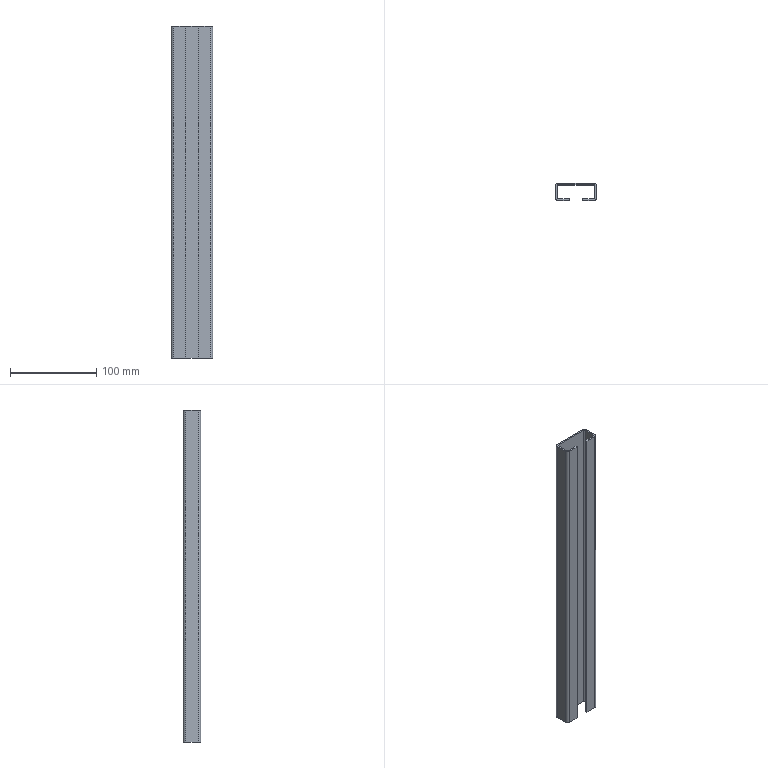Part | 1 solid | 38 faces | box 48 x 20 x 385 mm | volume 83596 mm3 | plane 30 | cylinder 8 | commonest cylinder face diameters 2 x4 6 x4
STEP:
#1=CARTESIAN_POINT('',(-24.,-17.,192.5));
#2=VERTEX_POINT('',#1);
#3=CARTESIAN_POINT('',(-22.,-17.,192.5));
#4=VERTEX_POINT('',#3);
#5=CARTESIAN_POINT('',(-24.,-17.,192.5));
#6=DIRECTION('',(1.,0.,0.));
#7=VECTOR('',#6,1000.);
#8=LINE('',#5,#7);
#9=EDGE_CURVE('',#2,#4,#8,.T.);
#10=ORIENTED_EDGE('',*,*,#9,.F.);
#11=CARTESIAN_POINT('',(-21.,-20.,192.5));
#12=VERTEX_POINT('',#11);
#13=CARTESIAN_POINT('',(-21.,-17.,192.5));
#14=DIRECTION('',(0.,0.,-1.));
#15=DIRECTION('',(1.,0.,0.));
#16=AXIS2_PLACEMENT_3D('',#13,#14,#15);
#17=CIRCLE('',#16,3.);
#18=EDGE_CURVE('',#12,#2,#17,.T.);
#19=ORIENTED_EDGE('',*,*,#18,.F.);
#20=CARTESIAN_POINT('',(-21.,-18.,192.5));
#21=VERTEX_POINT('',#20);
#22=CARTESIAN_POINT('',(-21.,-18.,192.5));
#23=DIRECTION('',(0.,-1.,0.));
#24=VECTOR('',#23,1000.);
#25=LINE('',#22,#24);
#26=EDGE_CURVE('',#21,#12,#25,.T.);
#27=ORIENTED_EDGE('',*,*,#26,.F.);
#28=CARTESIAN_POINT('',(-21.,-17.,192.5));
#29=DIRECTION('',(0.,0.,-1.));
#30=DIRECTION('',(1.,0.,0.));
#31=AXIS2_PLACEMENT_3D('',#28,#29,#30);
#32=CIRCLE('',#31,1.);
#33=EDGE_CURVE('',#21,#4,#32,.T.);
#34=ORIENTED_EDGE('',*,*,#33,.T.);
#35=EDGE_LOOP('',(#10,#19,#27,#34));
#36=FACE_OUTER_BOUND('',#35,.T.);
#37=CARTESIAN_POINT('',(-24.,-17.,192.5));
#38=DIRECTION('',(0.,0.,1.));
#39=DIRECTION('',(1.,0.,0.));
#40=AXIS2_PLACEMENT_3D('',#37,#38,#39);
#41=PLANE('',#40);
#42=ADVANCED_FACE('',(#36),#41,.T.);
#43=CARTESIAN_POINT('',(-24.,-3.,192.5));
#44=VERTEX_POINT('',#43);
#45=CARTESIAN_POINT('',(-24.,-20.,192.5));
#46=DIRECTION('',(0.,1.,0.));
#47=VECTOR('',#46,1000.);
#48=LINE('',#45,#47);
#49=EDGE_CURVE('',#2,#44,#48,.T.);
#50=ORIENTED_EDGE('',*,*,#49,.F.);
#51=ORIENTED_EDGE('',*,*,#9,.T.);
#52=CARTESIAN_POINT('',(-22.,-3.,192.5));
#53=VERTEX_POINT('',#52);
#54=CARTESIAN_POINT('',(-22.,-20.,192.5));
#55=DIRECTION('',(0.,1.,0.));
#56=VECTOR('',#55,1000.);
#57=LINE('',#54,#56);
#58=EDGE_CURVE('',#4,#53,#57,.T.);
#59=ORIENTED_EDGE('',*,*,#58,.T.);
#60=CARTESIAN_POINT('',(-22.,-3.,192.5));
#61=DIRECTION('',(-1.,0.,0.));
#62=VECTOR('',#61,1000.);
#63=LINE('',#60,#62);
#64=EDGE_CURVE('',#53,#44,#63,.T.);
#65=ORIENTED_EDGE('',*,*,#64,.T.);
#66=EDGE_LOOP('',(#50,#51,#59,#65));
#67=FACE_OUTER_BOUND('',#66,.T.);
#68=CARTESIAN_POINT('',(-21.,-18.,192.5));
#69=DIRECTION('',(0.,0.,1.));
#70=DIRECTION('',(1.,0.,0.));
#71=AXIS2_PLACEMENT_3D('',#68,#69,#70);
#72=PLANE('',#71);
#73=ADVANCED_FACE('',(#67),#72,.T.);
#74=CARTESIAN_POINT('',(-21.,-20.,-192.5));
#75=VERTEX_POINT('',#74);
#76=CARTESIAN_POINT('',(-21.,-18.,-192.5));
#77=VERTEX_POINT('',#76);
#78=CARTESIAN_POINT('',(-21.,-20.,-192.5));
#79=DIRECTION('',(0.,1.,0.));
#80=VECTOR('',#79,1000.);
#81=LINE('',#78,#80);
#82=EDGE_CURVE('',#75,#77,#81,.T.);
#83=ORIENTED_EDGE('',*,*,#82,.F.);
#84=CARTESIAN_POINT('',(-24.,-17.,-192.5));
#85=VERTEX_POINT('',#84);
#86=CARTESIAN_POINT('',(-21.,-17.,-192.5));
#87=DIRECTION('',(0.,0.,-1.));
#88=DIRECTION('',(1.,0.,0.));
#89=AXIS2_PLACEMENT_3D('',#86,#87,#88);
#90=CIRCLE('',#89,3.);
#91=EDGE_CURVE('',#75,#85,#90,.T.);
#92=ORIENTED_EDGE('',*,*,#91,.T.);
#93=CARTESIAN_POINT('',(-22.,-17.,-192.5));
#94=VERTEX_POINT('',#93);
#95=CARTESIAN_POINT('',(-22.,-17.,-192.5));
#96=DIRECTION('',(-1.,0.,0.));
#97=VECTOR('',#96,1000.);
#98=LINE('',#95,#97);
#99=EDGE_CURVE('',#94,#85,#98,.T.);
#100=ORIENTED_EDGE('',*,*,#99,.F.);
#101=CARTESIAN_POINT('',(-21.,-17.,-192.5));
#102=DIRECTION('',(0.,0.,-1.));
#103=DIRECTION('',(1.,0.,0.));
#104=AXIS2_PLACEMENT_3D('',#101,#102,#103);
#105=CIRCLE('',#104,1.);
#106=EDGE_CURVE('',#77,#94,#105,.T.);
#107=ORIENTED_EDGE('',*,*,#106,.F.);
#108=EDGE_LOOP('',(#83,#92,#100,#107));
#109=FACE_OUTER_BOUND('',#108,.T.);
#110=CARTESIAN_POINT('',(-21.,-20.,-192.5));
#111=DIRECTION('',(0.,0.,-1.));
#112=DIRECTION('',(-1.,0.,0.));
#113=AXIS2_PLACEMENT_3D('',#110,#111,#112);
#114=PLANE('',#113);
#115=ADVANCED_FACE('',(#109),#114,.T.);
#116=CARTESIAN_POINT('',(-8.,-20.,-192.5));
#117=VERTEX_POINT('',#116);
#118=CARTESIAN_POINT('',(-8.,-20.,-192.5));
#119=DIRECTION('',(-1.,0.,0.));
#120=VECTOR('',#119,1000.);
#121=LINE('',#118,#120);
#122=EDGE_CURVE('',#117,#75,#121,.T.);
#123=ORIENTED_EDGE('',*,*,#122,.T.);
#124=ORIENTED_EDGE('',*,*,#82,.T.);
#125=CARTESIAN_POINT('',(-8.,-18.,-192.5));
#126=VERTEX_POINT('',#125);
#127=CARTESIAN_POINT('',(-8.,-18.,-192.5));
#128=DIRECTION('',(-1.,0.,0.));
#129=VECTOR('',#128,1000.);
#130=LINE('',#127,#129);
#131=EDGE_CURVE('',#126,#77,#130,.T.);
#132=ORIENTED_EDGE('',*,*,#131,.F.);
#133=CARTESIAN_POINT('',(-8.,-18.,-192.5));
#134=DIRECTION('',(0.,-1.,0.));
#135=VECTOR('',#134,1000.);
#136=LINE('',#133,#135);
#137=EDGE_CURVE('',#126,#117,#136,.T.);
#138=ORIENTED_EDGE('',*,*,#137,.T.);
#139=EDGE_LOOP('',(#123,#124,#132,#138));
#140=FACE_OUTER_BOUND('',#139,.T.);
#141=CARTESIAN_POINT('',(-22.,-17.,-192.5));
#142=DIRECTION('',(0.,0.,-1.));
#143=DIRECTION('',(-1.,0.,0.));
#144=AXIS2_PLACEMENT_3D('',#141,#142,#143);
#145=PLANE('',#144);
#146=ADVANCED_FACE('',(#140),#145,.T.);
#147=CARTESIAN_POINT('',(-21.,0.,192.5));
#148=VERTEX_POINT('',#147);
#149=CARTESIAN_POINT('',(-21.,-2.,192.5));
#150=VERTEX_POINT('',#149);
#151=CARTESIAN_POINT('',(-21.,0.,192.5));
#152=DIRECTION('',(0.,-1.,0.));
#153=VECTOR('',#152,1000.);
#154=LINE('',#151,#153);
#155=EDGE_CURVE('',#148,#150,#154,.T.);
#156=ORIENTED_EDGE('',*,*,#155,.F.);
#157=CARTESIAN_POINT('',(-21.,-3.,192.5));
#158=DIRECTION('',(0.,0.,-1.));
#159=DIRECTION('',(1.,0.,0.));
#160=AXIS2_PLACEMENT_3D('',#157,#158,#159);
#161=CIRCLE('',#160,3.);
#162=EDGE_CURVE('',#44,#148,#161,.T.);
#163=ORIENTED_EDGE('',*,*,#162,.F.);
#164=ORIENTED_EDGE('',*,*,#64,.F.);
#165=CARTESIAN_POINT('',(-21.,-3.,192.5));
#166=DIRECTION('',(0.,0.,-1.));
#167=DIRECTION('',(1.,0.,0.));
#168=AXIS2_PLACEMENT_3D('',#165,#166,#167);
#169=CIRCLE('',#168,1.);
#170=EDGE_CURVE('',#53,#150,#169,.T.);
#171=ORIENTED_EDGE('',*,*,#170,.T.);
#172=EDGE_LOOP('',(#156,#163,#164,#171));
#173=FACE_OUTER_BOUND('',#172,.T.);
#174=CARTESIAN_POINT('',(-21.,0.,192.5));
#175=DIRECTION('',(0.,0.,1.));
#176=DIRECTION('',(1.,0.,0.));
#177=AXIS2_PLACEMENT_3D('',#174,#175,#176);
#178=PLANE('',#177);
#179=ADVANCED_FACE('',(#173),#178,.T.);
#180=CARTESIAN_POINT('',(21.,0.,192.5));
#181=VERTEX_POINT('',#180);
#182=CARTESIAN_POINT('',(-24.,0.,192.5));
#183=DIRECTION('',(1.,0.,0.));
#184=VECTOR('',#183,1000.);
#185=LINE('',#182,#184);
#186=EDGE_CURVE('',#148,#181,#185,.T.);
#187=ORIENTED_EDGE('',*,*,#186,.F.);
#188=ORIENTED_EDGE('',*,*,#155,.T.);
#189=CARTESIAN_POINT('',(21.,-2.,192.5));
#190=VERTEX_POINT('',#189);
#191=CARTESIAN_POINT('',(-24.,-2.,192.5));
#192=DIRECTION('',(1.,0.,0.));
#193=VECTOR('',#192,1000.);
#194=LINE('',#191,#193);
#195=EDGE_CURVE('',#150,#190,#194,.T.);
#196=ORIENTED_EDGE('',*,*,#195,.T.);
#197=CARTESIAN_POINT('',(21.,-2.,192.5));
#198=DIRECTION('',(0.,1.,0.));
#199=VECTOR('',#198,1000.);
#200=LINE('',#197,#199);
#201=EDGE_CURVE('',#190,#181,#200,.T.);
#202=ORIENTED_EDGE('',*,*,#201,.T.);
#203=EDGE_LOOP('',(#187,#188,#196,#202));
#204=FACE_OUTER_BOUND('',#203,.T.);
#205=CARTESIAN_POINT('',(-22.,-3.,192.5));
#206=DIRECTION('',(0.,0.,1.));
#207=DIRECTION('',(1.,0.,0.));
#208=AXIS2_PLACEMENT_3D('',#205,#206,#207);
#209=PLANE('',#208);
#210=ADVANCED_FACE('',(#204),#209,.T.);
#211=CARTESIAN_POINT('',(-24.,-3.,-192.5));
#212=VERTEX_POINT('',#211);
#213=CARTESIAN_POINT('',(-22.,-3.,-192.5));
#214=VERTEX_POINT('',#213);
#215=CARTESIAN_POINT('',(-24.,-3.,-192.5));
#216=DIRECTION('',(1.,0.,0.));
#217=VECTOR('',#216,1000.);
#218=LINE('',#215,#217);
#219=EDGE_CURVE('',#212,#214,#218,.T.);
#220=ORIENTED_EDGE('',*,*,#219,.F.);
#221=CARTESIAN_POINT('',(-21.,0.,-192.5));
#222=VERTEX_POINT('',#221);
#223=CARTESIAN_POINT('',(-21.,-3.,-192.5));
#224=DIRECTION('',(0.,0.,-1.));
#225=DIRECTION('',(1.,0.,0.));
#226=AXIS2_PLACEMENT_3D('',#223,#224,#225);
#227=CIRCLE('',#226,3.);
#228=EDGE_CURVE('',#212,#222,#227,.T.);
#229=ORIENTED_EDGE('',*,*,#228,.T.);
#230=CARTESIAN_POINT('',(-21.,-2.,-192.5));
#231=VERTEX_POINT('',#230);
#232=CARTESIAN_POINT('',(-21.,-2.,-192.5));
#233=DIRECTION('',(0.,1.,0.));
#234=VECTOR('',#233,1000.);
#235=LINE('',#232,#234);
#236=EDGE_CURVE('',#231,#222,#235,.T.);
#237=ORIENTED_EDGE('',*,*,#236,.F.);
#238=CARTESIAN_POINT('',(-21.,-3.,-192.5));
#239=DIRECTION('',(0.,0.,-1.));
#240=DIRECTION('',(1.,0.,0.));
#241=AXIS2_PLACEMENT_3D('',#238,#239,#240);
#242=CIRCLE('',#241,1.);
#243=EDGE_CURVE('',#214,#231,#242,.T.);
#244=ORIENTED_EDGE('',*,*,#243,.F.);
#245=EDGE_LOOP('',(#220,#229,#237,#244));
#246=FACE_OUTER_BOUND('',#245,.T.);
#247=CARTESIAN_POINT('',(-24.,-3.,-192.5));
#248=DIRECTION('',(0.,0.,-1.));
#249=DIRECTION('',(-1.,0.,0.));
#250=AXIS2_PLACEMENT_3D('',#247,#248,#249);
#251=PLANE('',#250);
#252=ADVANCED_FACE('',(#246),#251,.T.);
#253=CARTESIAN_POINT('',(-24.,-20.,-192.5));
#254=DIRECTION('',(0.,1.,0.));
#255=VECTOR('',#254,1000.);
#256=LINE('',#253,#255);
#257=EDGE_CURVE('',#85,#212,#256,.T.);
#258=ORIENTED_EDGE('',*,*,#257,.T.);
#259=ORIENTED_EDGE('',*,*,#219,.T.);
#260=CARTESIAN_POINT('',(-22.,-20.,-192.5));
#261=DIRECTION('',(0.,1.,0.));
#262=VECTOR('',#261,1000.);
#263=LINE('',#260,#262);
#264=EDGE_CURVE('',#94,#214,#263,.T.);
#265=ORIENTED_EDGE('',*,*,#264,.F.);
#266=ORIENTED_EDGE('',*,*,#99,.T.);
#267=EDGE_LOOP('',(#258,#259,#265,#266));
#268=FACE_OUTER_BOUND('',#267,.T.);
#269=CARTESIAN_POINT('',(-21.,-2.,-192.5));
#270=DIRECTION('',(0.,0.,-1.));
#271=DIRECTION('',(-1.,0.,0.));
#272=AXIS2_PLACEMENT_3D('',#269,#270,#271);
#273=PLANE('',#272);
#274=ADVANCED_FACE('',(#268),#273,.T.);
#275=CARTESIAN_POINT('',(24.,-3.,192.5));
#276=VERTEX_POINT('',#275);
#277=CARTESIAN_POINT('',(22.,-3.,192.5));
#278=VERTEX_POINT('',#277);
#279=CARTESIAN_POINT('',(24.,-3.,192.5));
#280=DIRECTION('',(-1.,0.,0.));
#281=VECTOR('',#280,1000.);
#282=LINE('',#279,#281);
#283=EDGE_CURVE('',#276,#278,#282,.T.);
#284=ORIENTED_EDGE('',*,*,#283,.F.);
#285=CARTESIAN_POINT('',(21.,-3.,192.5));
#286=DIRECTION('',(0.,0.,-1.));
#287=DIRECTION('',(1.,0.,0.));
#288=AXIS2_PLACEMENT_3D('',#285,#286,#287);
#289=CIRCLE('',#288,3.);
#290=EDGE_CURVE('',#181,#276,#289,.T.);
#291=ORIENTED_EDGE('',*,*,#290,.F.);
#292=ORIENTED_EDGE('',*,*,#201,.F.);
#293=CARTESIAN_POINT('',(21.,-3.,192.5));
#294=DIRECTION('',(0.,0.,-1.));
#295=DIRECTION('',(1.,0.,0.));
#296=AXIS2_PLACEMENT_3D('',#293,#294,#295);
#297=CIRCLE('',#296,1.);
#298=EDGE_CURVE('',#190,#278,#297,.T.);
#299=ORIENTED_EDGE('',*,*,#298,.T.);
#300=EDGE_LOOP('',(#284,#291,#292,#299));
#301=FACE_OUTER_BOUND('',#300,.T.);
#302=CARTESIAN_POINT('',(24.,-3.,192.5));
#303=DIRECTION('',(0.,0.,1.));
#304=DIRECTION('',(1.,0.,0.));
#305=AXIS2_PLACEMENT_3D('',#302,#303,#304);
#306=PLANE('',#305);
#307=ADVANCED_FACE('',(#301),#306,.T.);
#308=CARTESIAN_POINT('',(24.,-17.,192.5));
#309=VERTEX_POINT('',#308);
#310=CARTESIAN_POINT('',(24.,0.,192.5));
#311=DIRECTION('',(0.,-1.,0.));
#312=VECTOR('',#311,1000.);
#313=LINE('',#310,#312);
#314=EDGE_CURVE('',#276,#309,#313,.T.);
#315=ORIENTED_EDGE('',*,*,#314,.F.);
#316=ORIENTED_EDGE('',*,*,#283,.T.);
#317=CARTESIAN_POINT('',(22.,-17.,192.5));
#318=VERTEX_POINT('',#317);
#319=CARTESIAN_POINT('',(22.,0.,192.5));
#320=DIRECTION('',(0.,-1.,0.));
#321=VECTOR('',#320,1000.);
#322=LINE('',#319,#321);
#323=EDGE_CURVE('',#278,#318,#322,.T.);
#324=ORIENTED_EDGE('',*,*,#323,.T.);
#325=CARTESIAN_POINT('',(22.,-17.,192.5));
#326=DIRECTION('',(1.,0.,0.));
#327=VECTOR('',#326,1000.);
#328=LINE('',#325,#327);
#329=EDGE_CURVE('',#318,#309,#328,.T.);
#330=ORIENTED_EDGE('',*,*,#329,.T.);
#331=EDGE_LOOP('',(#315,#316,#324,#330));
#332=FACE_OUTER_BOUND('',#331,.T.);
#333=CARTESIAN_POINT('',(21.,-2.,192.5));
#334=DIRECTION('',(0.,0.,1.));
#335=DIRECTION('',(1.,0.,0.));
#336=AXIS2_PLACEMENT_3D('',#333,#334,#335);
#337=PLANE('',#336);
#338=ADVANCED_FACE('',(#332),#337,.T.);
#339=CARTESIAN_POINT('',(21.,0.,-192.5));
#340=VERTEX_POINT('',#339);
#341=CARTESIAN_POINT('',(21.,-2.,-192.5));
#342=VERTEX_POINT('',#341);
#343=CARTESIAN_POINT('',(21.,0.,-192.5));
#344=DIRECTION('',(0.,-1.,0.));
#345=VECTOR('',#344,1000.);
#346=LINE('',#343,#345);
#347=EDGE_CURVE('',#340,#342,#346,.T.);
#348=ORIENTED_EDGE('',*,*,#347,.F.);
#349=CARTESIAN_POINT('',(24.,-3.,-192.5));
#350=VERTEX_POINT('',#349);
#351=CARTESIAN_POINT('',(21.,-3.,-192.5));
#352=DIRECTION('',(0.,0.,-1.));
#353=DIRECTION('',(1.,0.,0.));
#354=AXIS2_PLACEMENT_3D('',#351,#352,#353);
#355=CIRCLE('',#354,3.);
#356=EDGE_CURVE('',#340,#350,#355,.T.);
#357=ORIENTED_EDGE('',*,*,#356,.T.);
#358=CARTESIAN_POINT('',(22.,-3.,-192.5));
#359=VERTEX_POINT('',#358);
#360=CARTESIAN_POINT('',(22.,-3.,-192.5));
#361=DIRECTION('',(1.,0.,0.));
#362=VECTOR('',#361,1000.);
#363=LINE('',#360,#362);
#364=EDGE_CURVE('',#359,#350,#363,.T.);
#365=ORIENTED_EDGE('',*,*,#364,.F.);
#366=CARTESIAN_POINT('',(21.,-3.,-192.5));
#367=DIRECTION('',(0.,0.,-1.));
#368=DIRECTION('',(1.,0.,0.));
#369=AXIS2_PLACEMENT_3D('',#366,#367,#368);
#370=CIRCLE('',#369,1.);
#371=EDGE_CURVE('',#342,#359,#370,.T.);
#372=ORIENTED_EDGE('',*,*,#371,.F.);
#373=EDGE_LOOP('',(#348,#357,#365,#372));
#374=FACE_OUTER_BOUND('',#373,.T.);
#375=CARTESIAN_POINT('',(21.,0.,-192.5));
#376=DIRECTION('',(0.,0.,-1.));
#377=DIRECTION('',(-1.,0.,0.));
#378=AXIS2_PLACEMENT_3D('',#375,#376,#377);
#379=PLANE('',#378);
#380=ADVANCED_FACE('',(#374),#379,.T.);
#381=CARTESIAN_POINT('',(-24.,0.,-192.5));
#382=DIRECTION('',(1.,0.,0.));
#383=VECTOR('',#382,1000.);
#384=LINE('',#381,#383);
#385=EDGE_CURVE('',#222,#340,#384,.T.);
#386=ORIENTED_EDGE('',*,*,#385,.T.);
#387=ORIENTED_EDGE('',*,*,#347,.T.);
#388=CARTESIAN_POINT('',(-24.,-2.,-192.5));
#389=DIRECTION('',(1.,0.,0.));
#390=VECTOR('',#389,1000.);
#391=LINE('',#388,#390);
#392=EDGE_CURVE('',#231,#342,#391,.T.);
#393=ORIENTED_EDGE('',*,*,#392,.F.);
#394=ORIENTED_EDGE('',*,*,#236,.T.);
#395=EDGE_LOOP('',(#386,#387,#393,#394));
#396=FACE_OUTER_BOUND('',#395,.T.);
#397=CARTESIAN_POINT('',(22.,-3.,-192.5));
#398=DIRECTION('',(0.,0.,-1.));
#399=DIRECTION('',(-1.,0.,0.));
#400=AXIS2_PLACEMENT_3D('',#397,#398,#399);
#401=PLANE('',#400);
#402=ADVANCED_FACE('',(#396),#401,.T.);
#403=CARTESIAN_POINT('',(21.,-20.,192.5));
#404=VERTEX_POINT('',#403);
#405=CARTESIAN_POINT('',(21.,-18.,192.5));
#406=VERTEX_POINT('',#405);
#407=CARTESIAN_POINT('',(21.,-20.,192.5));
#408=DIRECTION('',(0.,1.,0.));
#409=VECTOR('',#408,1000.);
#410=LINE('',#407,#409);
#411=EDGE_CURVE('',#404,#406,#410,.T.);
#412=ORIENTED_EDGE('',*,*,#411,.F.);
#413=CARTESIAN_POINT('',(21.,-17.,192.5));
#414=DIRECTION('',(0.,0.,-1.));
#415=DIRECTION('',(1.,0.,0.));
#416=AXIS2_PLACEMENT_3D('',#413,#414,#415);
#417=CIRCLE('',#416,3.);
#418=EDGE_CURVE('',#309,#404,#417,.T.);
#419=ORIENTED_EDGE('',*,*,#418,.F.);
#420=ORIENTED_EDGE('',*,*,#329,.F.);
#421=CARTESIAN_POINT('',(21.,-17.,192.5));
#422=DIRECTION('',(0.,0.,-1.));
#423=DIRECTION('',(1.,0.,0.));
#424=AXIS2_PLACEMENT_3D('',#421,#422,#423);
#425=CIRCLE('',#424,1.);
#426=EDGE_CURVE('',#318,#406,#425,.T.);
#427=ORIENTED_EDGE('',*,*,#426,.T.);
#428=EDGE_LOOP('',(#412,#419,#420,#427));
#429=FACE_OUTER_BOUND('',#428,.T.);
#430=CARTESIAN_POINT('',(21.,-20.,192.5));
#431=DIRECTION('',(0.,0.,1.));
#432=DIRECTION('',(1.,0.,0.));
#433=AXIS2_PLACEMENT_3D('',#430,#431,#432);
#434=PLANE('',#433);
#435=ADVANCED_FACE('',(#429),#434,.T.);
#436=CARTESIAN_POINT('',(8.,-20.,192.5));
#437=VERTEX_POINT('',#436);
#438=CARTESIAN_POINT('',(24.,-20.,192.5));
#439=DIRECTION('',(-1.,0.,0.));
#440=VECTOR('',#439,1000.);
#441=LINE('',#438,#440);
#442=EDGE_CURVE('',#404,#437,#441,.T.);
#443=ORIENTED_EDGE('',*,*,#442,.F.);
#444=ORIENTED_EDGE('',*,*,#411,.T.);
#445=CARTESIAN_POINT('',(8.,-18.,192.5));
#446=VERTEX_POINT('',#445);
#447=CARTESIAN_POINT('',(24.,-18.,192.5));
#448=DIRECTION('',(-1.,0.,0.));
#449=VECTOR('',#448,1000.);
#450=LINE('',#447,#449);
#451=EDGE_CURVE('',#406,#446,#450,.T.);
#452=ORIENTED_EDGE('',*,*,#451,.T.);
#453=CARTESIAN_POINT('',(8.,-20.,192.5));
#454=DIRECTION('',(0.,1.,0.));
#455=VECTOR('',#454,1000.);
#456=LINE('',#453,#455);
#457=EDGE_CURVE('',#437,#446,#456,.T.);
#458=ORIENTED_EDGE('',*,*,#457,.F.);
#459=EDGE_LOOP('',(#443,#444,#452,#458));
#460=FACE_OUTER_BOUND('',#459,.T.);
#461=CARTESIAN_POINT('',(22.,-17.,192.5));
#462=DIRECTION('',(0.,0.,1.));
#463=DIRECTION('',(1.,0.,0.));
#464=AXIS2_PLACEMENT_3D('',#461,#462,#463);
#465=PLANE('',#464);
#466=ADVANCED_FACE('',(#460),#465,.T.);
#467=CARTESIAN_POINT('',(24.,-17.,-192.5));
#468=VERTEX_POINT('',#467);
#469=CARTESIAN_POINT('',(22.,-17.,-192.5));
#470=VERTEX_POINT('',#469);
#471=CARTESIAN_POINT('',(24.,-17.,-192.5));
#472=DIRECTION('',(-1.,0.,0.));
#473=VECTOR('',#472,1000.);
#474=LINE('',#471,#473);
#475=EDGE_CURVE('',#468,#470,#474,.T.);
#476=ORIENTED_EDGE('',*,*,#475,.F.);
#477=CARTESIAN_POINT('',(21.,-20.,-192.5));
#478=VERTEX_POINT('',#477);
#479=CARTESIAN_POINT('',(21.,-17.,-192.5));
#480=DIRECTION('',(0.,0.,-1.));
#481=DIRECTION('',(1.,0.,0.));
#482=AXIS2_PLACEMENT_3D('',#479,#480,#481);
#483=CIRCLE('',#482,3.);
#484=EDGE_CURVE('',#468,#478,#483,.T.);
#485=ORIENTED_EDGE('',*,*,#484,.T.);
#486=CARTESIAN_POINT('',(21.,-18.,-192.5));
#487=VERTEX_POINT('',#486);
#488=CARTESIAN_POINT('',(21.,-18.,-192.5));
#489=DIRECTION('',(0.,-1.,0.));
#490=VECTOR('',#489,1000.);
#491=LINE('',#488,#490);
#492=EDGE_CURVE('',#487,#478,#491,.T.);
#493=ORIENTED_EDGE('',*,*,#492,.F.);
#494=CARTESIAN_POINT('',(21.,-17.,-192.5));
#495=DIRECTION('',(0.,0.,-1.));
#496=DIRECTION('',(1.,0.,0.));
#497=AXIS2_PLACEMENT_3D('',#494,#495,#496);
#498=CIRCLE('',#497,1.);
#499=EDGE_CURVE('',#470,#487,#498,.T.);
#500=ORIENTED_EDGE('',*,*,#499,.F.);
#501=EDGE_LOOP('',(#476,#485,#493,#500));
#502=FACE_OUTER_BOUND('',#501,.T.);
#503=CARTESIAN_POINT('',(24.,-17.,-192.5));
#504=DIRECTION('',(0.,0.,-1.));
#505=DIRECTION('',(-1.,0.,0.));
#506=AXIS2_PLACEMENT_3D('',#503,#504,#505);
#507=PLANE('',#506);
#508=ADVANCED_FACE('',(#502),#507,.T.);
#509=CARTESIAN_POINT('',(24.,0.,-192.5));
#510=DIRECTION('',(0.,-1.,0.));
#511=VECTOR('',#510,1000.);
#512=LINE('',#509,#511);
#513=EDGE_CURVE('',#350,#468,#512,.T.);
#514=ORIENTED_EDGE('',*,*,#513,.T.);
#515=ORIENTED_EDGE('',*,*,#475,.T.);
#516=CARTESIAN_POINT('',(22.,0.,-192.5));
#517=DIRECTION('',(0.,-1.,0.));
#518=VECTOR('',#517,1000.);
#519=LINE('',#516,#518);
#520=EDGE_CURVE('',#359,#470,#519,.T.);
#521=ORIENTED_EDGE('',*,*,#520,.F.);
#522=ORIENTED_EDGE('',*,*,#364,.T.);
#523=EDGE_LOOP('',(#514,#515,#521,#522));
#524=FACE_OUTER_BOUND('',#523,.T.);
#525=CARTESIAN_POINT('',(21.,-18.,-192.5));
#526=DIRECTION('',(0.,0.,-1.));
#527=DIRECTION('',(-1.,0.,0.));
#528=AXIS2_PLACEMENT_3D('',#525,#526,#527);
#529=PLANE('',#528);
#530=ADVANCED_FACE('',(#524),#529,.T.);
#531=CARTESIAN_POINT('',(8.,-18.,-192.5));
#532=VERTEX_POINT('',#531);
#533=CARTESIAN_POINT('',(24.,-18.,-192.5));
#534=DIRECTION('',(-1.,0.,0.));
#535=VECTOR('',#534,1000.);
#536=LINE('',#533,#535);
#537=EDGE_CURVE('',#487,#532,#536,.T.);
#538=ORIENTED_EDGE('',*,*,#537,.T.);
#539=CARTESIAN_POINT('',(8.,-18.,192.5));
#540=DIRECTION('',(0.,0.,-1.));
#541=VECTOR('',#540,1000.);
#542=LINE('',#539,#541);
#543=EDGE_CURVE('',#446,#532,#542,.T.);
#544=ORIENTED_EDGE('',*,*,#543,.F.);
#545=ORIENTED_EDGE('',*,*,#451,.F.);
#546=CARTESIAN_POINT('',(21.,-18.,192.5));
#547=DIRECTION('',(0.,0.,-1.));
#548=VECTOR('',#547,1000.);
#549=LINE('',#546,#548);
#550=EDGE_CURVE('',#406,#487,#549,.T.);
#551=ORIENTED_EDGE('',*,*,#550,.T.);
#552=EDGE_LOOP('',(#538,#544,#545,#551));
#553=FACE_OUTER_BOUND('',#552,.T.);
#554=CARTESIAN_POINT('',(24.,-18.,192.5));
#555=DIRECTION('',(0.,-1.,0.));
#556=DIRECTION('',(1.,0.,0.));
#557=AXIS2_PLACEMENT_3D('',#554,#555,#556);
#558=PLANE('',#557);
#559=ADVANCED_FACE('',(#553),#558,.F.);
#560=CARTESIAN_POINT('',(8.,-20.,-192.5));
#561=VERTEX_POINT('',#560);
#562=CARTESIAN_POINT('',(8.,-20.,-192.5));
#563=DIRECTION('',(0.,1.,0.));
#564=VECTOR('',#563,1000.);
#565=LINE('',#562,#564);
#566=EDGE_CURVE('',#561,#532,#565,.T.);
#567=ORIENTED_EDGE('',*,*,#566,.F.);
#568=CARTESIAN_POINT('',(8.,-20.,192.5));
#569=DIRECTION('',(0.,0.,-1.));
#570=VECTOR('',#569,1000.);
#571=LINE('',#568,#570);
#572=EDGE_CURVE('',#437,#561,#571,.T.);
#573=ORIENTED_EDGE('',*,*,#572,.F.);
#574=ORIENTED_EDGE('',*,*,#457,.T.);
#575=ORIENTED_EDGE('',*,*,#543,.T.);
#576=EDGE_LOOP('',(#567,#573,#574,#575));
#577=FACE_OUTER_BOUND('',#576,.T.);
#578=CARTESIAN_POINT('',(8.,-20.,192.5));
#579=DIRECTION('',(-1.,0.,0.));
#580=DIRECTION('',(0.,0.,1.));
#581=AXIS2_PLACEMENT_3D('',#578,#579,#580);
#582=PLANE('',#581);
#583=ADVANCED_FACE('',(#577),#582,.T.);
#584=CARTESIAN_POINT('',(24.,-20.,-192.5));
#585=DIRECTION('',(-1.,0.,0.));
#586=VECTOR('',#585,1000.);
#587=LINE('',#584,#586);
#588=EDGE_CURVE('',#478,#561,#587,.T.);
#589=ORIENTED_EDGE('',*,*,#588,.F.);
#590=CARTESIAN_POINT('',(21.,-20.,192.5));
#591=DIRECTION('',(0.,0.,-1.));
#592=VECTOR('',#591,1000.);
#593=LINE('',#590,#592);
#594=EDGE_CURVE('',#404,#478,#593,.T.);
#595=ORIENTED_EDGE('',*,*,#594,.F.);
#596=ORIENTED_EDGE('',*,*,#442,.T.);
#597=ORIENTED_EDGE('',*,*,#572,.T.);
#598=EDGE_LOOP('',(#589,#595,#596,#597));
#599=FACE_OUTER_BOUND('',#598,.T.);
#600=CARTESIAN_POINT('',(24.,-20.,192.5));
#601=DIRECTION('',(0.,-1.,0.));
#602=DIRECTION('',(1.,0.,0.));
#603=AXIS2_PLACEMENT_3D('',#600,#601,#602);
#604=PLANE('',#603);
#605=ADVANCED_FACE('',(#599),#604,.T.);
#606=ORIENTED_EDGE('',*,*,#484,.F.);
#607=CARTESIAN_POINT('',(24.,-17.,192.5));
#608=DIRECTION('',(0.,0.,-1.));
#609=VECTOR('',#608,1000.);
#610=LINE('',#607,#609);
#611=EDGE_CURVE('',#309,#468,#610,.T.);
#612=ORIENTED_EDGE('',*,*,#611,.F.);
#613=ORIENTED_EDGE('',*,*,#418,.T.);
#614=ORIENTED_EDGE('',*,*,#594,.T.);
#615=EDGE_LOOP('',(#606,#612,#613,#614));
#616=FACE_OUTER_BOUND('',#615,.T.);
#617=CARTESIAN_POINT('',(21.,-17.,192.5));
#618=DIRECTION('',(0.,0.,-1.));
#619=DIRECTION('',(-1.,0.,0.));
#620=AXIS2_PLACEMENT_3D('',#617,#618,#619);
#621=CYLINDRICAL_SURFACE('',#620,3.);
#622=ADVANCED_FACE('',(#616),#621,.T.);
#623=ORIENTED_EDGE('',*,*,#513,.F.);
#624=CARTESIAN_POINT('',(24.,-3.,192.5));
#625=DIRECTION('',(0.,0.,-1.));
#626=VECTOR('',#625,1000.);
#627=LINE('',#624,#626);
#628=EDGE_CURVE('',#276,#350,#627,.T.);
#629=ORIENTED_EDGE('',*,*,#628,.F.);
#630=ORIENTED_EDGE('',*,*,#314,.T.);
#631=ORIENTED_EDGE('',*,*,#611,.T.);
#632=EDGE_LOOP('',(#623,#629,#630,#631));
#633=FACE_OUTER_BOUND('',#632,.T.);
#634=CARTESIAN_POINT('',(24.,0.,192.5));
#635=DIRECTION('',(1.,0.,0.));
#636=DIRECTION('',(0.,0.,-1.));
#637=AXIS2_PLACEMENT_3D('',#634,#635,#636);
#638=PLANE('',#637);
#639=ADVANCED_FACE('',(#633),#638,.T.);
#640=ORIENTED_EDGE('',*,*,#356,.F.);
#641=CARTESIAN_POINT('',(21.,0.,192.5));
#642=DIRECTION('',(0.,0.,-1.));
#643=VECTOR('',#642,1000.);
#644=LINE('',#641,#643);
#645=EDGE_CURVE('',#181,#340,#644,.T.);
#646=ORIENTED_EDGE('',*,*,#645,.F.);
#647=ORIENTED_EDGE('',*,*,#290,.T.);
#648=ORIENTED_EDGE('',*,*,#628,.T.);
#649=EDGE_LOOP('',(#640,#646,#647,#648));
#650=FACE_OUTER_BOUND('',#649,.T.);
#651=CARTESIAN_POINT('',(21.,-3.,192.5));
#652=DIRECTION('',(0.,0.,-1.));
#653=DIRECTION('',(-1.,0.,0.));
#654=AXIS2_PLACEMENT_3D('',#651,#652,#653);
#655=CYLINDRICAL_SURFACE('',#654,3.);
#656=ADVANCED_FACE('',(#650),#655,.T.);
#657=ORIENTED_EDGE('',*,*,#385,.F.);
#658=CARTESIAN_POINT('',(-21.,0.,192.5));
#659=DIRECTION('',(0.,0.,-1.));
#660=VECTOR('',#659,1000.);
#661=LINE('',#658,#660);
#662=EDGE_CURVE('',#148,#222,#661,.T.);
#663=ORIENTED_EDGE('',*,*,#662,.F.);
#664=ORIENTED_EDGE('',*,*,#186,.T.);
#665=ORIENTED_EDGE('',*,*,#645,.T.);
#666=EDGE_LOOP('',(#657,#663,#664,#665));
#667=FACE_OUTER_BOUND('',#666,.T.);
#668=CARTESIAN_POINT('',(-24.,0.,192.5));
#669=DIRECTION('',(0.,1.,0.));
#670=DIRECTION('',(0.,0.,1.));
#671=AXIS2_PLACEMENT_3D('',#668,#669,#670);
#672=PLANE('',#671);
#673=ADVANCED_FACE('',(#667),#672,.T.);
#674=ORIENTED_EDGE('',*,*,#228,.F.);
#675=CARTESIAN_POINT('',(-24.,-3.,192.5));
#676=DIRECTION('',(0.,0.,-1.));
#677=VECTOR('',#676,1000.);
#678=LINE('',#675,#677);
#679=EDGE_CURVE('',#44,#212,#678,.T.);
#680=ORIENTED_EDGE('',*,*,#679,.F.);
#681=ORIENTED_EDGE('',*,*,#162,.T.);
#682=ORIENTED_EDGE('',*,*,#662,.T.);
#683=EDGE_LOOP('',(#674,#680,#681,#682));
#684=FACE_OUTER_BOUND('',#683,.T.);
#685=CARTESIAN_POINT('',(-21.,-3.,192.5));
#686=DIRECTION('',(0.,0.,-1.));
#687=DIRECTION('',(-1.,0.,0.));
#688=AXIS2_PLACEMENT_3D('',#685,#686,#687);
#689=CYLINDRICAL_SURFACE('',#688,3.);
#690=ADVANCED_FACE('',(#684),#689,.T.);
#691=ORIENTED_EDGE('',*,*,#257,.F.);
#692=CARTESIAN_POINT('',(-24.,-17.,192.5));
#693=DIRECTION('',(0.,0.,-1.));
#694=VECTOR('',#693,1000.);
#695=LINE('',#692,#694);
#696=EDGE_CURVE('',#2,#85,#695,.T.);
#697=ORIENTED_EDGE('',*,*,#696,.F.);
#698=ORIENTED_EDGE('',*,*,#49,.T.);
#699=ORIENTED_EDGE('',*,*,#679,.T.);
#700=EDGE_LOOP('',(#691,#697,#698,#699));
#701=FACE_OUTER_BOUND('',#700,.T.);
#702=CARTESIAN_POINT('',(-24.,-20.,192.5));
#703=DIRECTION('',(-1.,0.,0.));
#704=DIRECTION('',(0.,0.,1.));
#705=AXIS2_PLACEMENT_3D('',#702,#703,#704);
#706=PLANE('',#705);
#707=ADVANCED_FACE('',(#701),#706,.T.);
#708=ORIENTED_EDGE('',*,*,#91,.F.);
#709=CARTESIAN_POINT('',(-21.,-20.,192.5));
#710=DIRECTION('',(0.,0.,-1.));
#711=VECTOR('',#710,1000.);
#712=LINE('',#709,#711);
#713=EDGE_CURVE('',#12,#75,#712,.T.);
#714=ORIENTED_EDGE('',*,*,#713,.F.);
#715=ORIENTED_EDGE('',*,*,#18,.T.);
#716=ORIENTED_EDGE('',*,*,#696,.T.);
#717=EDGE_LOOP('',(#708,#714,#715,#716));
#718=FACE_OUTER_BOUND('',#717,.T.);
#719=CARTESIAN_POINT('',(-21.,-17.,192.5));
#720=DIRECTION('',(0.,0.,-1.));
#721=DIRECTION('',(-1.,0.,0.));
#722=AXIS2_PLACEMENT_3D('',#719,#720,#721);
#723=CYLINDRICAL_SURFACE('',#722,3.);
#724=ADVANCED_FACE('',(#718),#723,.T.);
#725=ORIENTED_EDGE('',*,*,#122,.F.);
#726=CARTESIAN_POINT('',(-8.,-20.,192.5));
#727=VERTEX_POINT('',#726);
#728=CARTESIAN_POINT('',(-8.,-20.,192.5));
#729=DIRECTION('',(0.,0.,-1.));
#730=VECTOR('',#729,1000.);
#731=LINE('',#728,#730);
#732=EDGE_CURVE('',#727,#117,#731,.T.);
#733=ORIENTED_EDGE('',*,*,#732,.F.);
#734=CARTESIAN_POINT('',(-8.,-20.,192.5));
#735=DIRECTION('',(-1.,0.,0.));
#736=VECTOR('',#735,1000.);
#737=LINE('',#734,#736);
#738=EDGE_CURVE('',#727,#12,#737,.T.);
#739=ORIENTED_EDGE('',*,*,#738,.T.);
#740=ORIENTED_EDGE('',*,*,#713,.T.);
#741=EDGE_LOOP('',(#725,#733,#739,#740));
#742=FACE_OUTER_BOUND('',#741,.T.);
#743=CARTESIAN_POINT('',(-8.,-20.,192.5));
#744=DIRECTION('',(0.,-1.,0.));
#745=DIRECTION('',(1.,0.,0.));
#746=AXIS2_PLACEMENT_3D('',#743,#744,#745);
#747=PLANE('',#746);
#748=ADVANCED_FACE('',(#742),#747,.T.);
#749=ORIENTED_EDGE('',*,*,#137,.F.);
#750=CARTESIAN_POINT('',(-8.,-18.,192.5));
#751=VERTEX_POINT('',#750);
#752=CARTESIAN_POINT('',(-8.,-18.,192.5));
#753=DIRECTION('',(0.,0.,-1.));
#754=VECTOR('',#753,1000.);
#755=LINE('',#752,#754);
#756=EDGE_CURVE('',#751,#126,#755,.T.);
#757=ORIENTED_EDGE('',*,*,#756,.F.);
#758=CARTESIAN_POINT('',(-8.,-18.,192.5));
#759=DIRECTION('',(0.,-1.,0.));
#760=VECTOR('',#759,1000.);
#761=LINE('',#758,#760);
#762=EDGE_CURVE('',#751,#727,#761,.T.);
#763=ORIENTED_EDGE('',*,*,#762,.T.);
#764=ORIENTED_EDGE('',*,*,#732,.T.);
#765=EDGE_LOOP('',(#749,#757,#763,#764));
#766=FACE_OUTER_BOUND('',#765,.T.);
#767=CARTESIAN_POINT('',(-8.,-18.,192.5));
#768=DIRECTION('',(1.,0.,0.));
#769=DIRECTION('',(0.,0.,-1.));
#770=AXIS2_PLACEMENT_3D('',#767,#768,#769);
#771=PLANE('',#770);
#772=ADVANCED_FACE('',(#766),#771,.T.);
#773=ORIENTED_EDGE('',*,*,#131,.T.);
#774=CARTESIAN_POINT('',(-21.,-18.,192.5));
#775=DIRECTION('',(0.,0.,-1.));
#776=VECTOR('',#775,1000.);
#777=LINE('',#774,#776);
#778=EDGE_CURVE('',#21,#77,#777,.T.);
#779=ORIENTED_EDGE('',*,*,#778,.F.);
#780=CARTESIAN_POINT('',(-8.,-18.,192.5));
#781=DIRECTION('',(-1.,0.,0.));
#782=VECTOR('',#781,1000.);
#783=LINE('',#780,#782);
#784=EDGE_CURVE('',#751,#21,#783,.T.);
#785=ORIENTED_EDGE('',*,*,#784,.F.);
#786=ORIENTED_EDGE('',*,*,#756,.T.);
#787=EDGE_LOOP('',(#773,#779,#785,#786));
#788=FACE_OUTER_BOUND('',#787,.T.);
#789=CARTESIAN_POINT('',(-8.,-18.,192.5));
#790=DIRECTION('',(0.,-1.,0.));
#791=DIRECTION('',(1.,0.,0.));
#792=AXIS2_PLACEMENT_3D('',#789,#790,#791);
#793=PLANE('',#792);
#794=ADVANCED_FACE('',(#788),#793,.F.);
#795=ORIENTED_EDGE('',*,*,#106,.T.);
#796=CARTESIAN_POINT('',(-22.,-17.,192.5));
#797=DIRECTION('',(0.,0.,-1.));
#798=VECTOR('',#797,1000.);
#799=LINE('',#796,#798);
#800=EDGE_CURVE('',#4,#94,#799,.T.);
#801=ORIENTED_EDGE('',*,*,#800,.F.);
#802=ORIENTED_EDGE('',*,*,#33,.F.);
#803=ORIENTED_EDGE('',*,*,#778,.T.);
#804=EDGE_LOOP('',(#795,#801,#802,#803));
#805=FACE_OUTER_BOUND('',#804,.T.);
#806=CARTESIAN_POINT('',(-21.,-17.,192.5));
#807=DIRECTION('',(0.,0.,-1.));
#808=DIRECTION('',(-1.,0.,0.));
#809=AXIS2_PLACEMENT_3D('',#806,#807,#808);
#810=CYLINDRICAL_SURFACE('',#809,1.);
#811=ADVANCED_FACE('',(#805),#810,.F.);
#812=ORIENTED_EDGE('',*,*,#264,.T.);
#813=CARTESIAN_POINT('',(-22.,-3.,192.5));
#814=DIRECTION('',(0.,0.,-1.));
#815=VECTOR('',#814,1000.);
#816=LINE('',#813,#815);
#817=EDGE_CURVE('',#53,#214,#816,.T.);
#818=ORIENTED_EDGE('',*,*,#817,.F.);
#819=ORIENTED_EDGE('',*,*,#58,.F.);
#820=ORIENTED_EDGE('',*,*,#800,.T.);
#821=EDGE_LOOP('',(#812,#818,#819,#820));
#822=FACE_OUTER_BOUND('',#821,.T.);
#823=CARTESIAN_POINT('',(-22.,-20.,192.5));
#824=DIRECTION('',(-1.,0.,0.));
#825=DIRECTION('',(0.,0.,1.));
#826=AXIS2_PLACEMENT_3D('',#823,#824,#825);
#827=PLANE('',#826);
#828=ADVANCED_FACE('',(#822),#827,.F.);
#829=ORIENTED_EDGE('',*,*,#243,.T.);
#830=CARTESIAN_POINT('',(-21.,-2.,192.5));
#831=DIRECTION('',(0.,0.,-1.));
#832=VECTOR('',#831,1000.);
#833=LINE('',#830,#832);
#834=EDGE_CURVE('',#150,#231,#833,.T.);
#835=ORIENTED_EDGE('',*,*,#834,.F.);
#836=ORIENTED_EDGE('',*,*,#170,.F.);
#837=ORIENTED_EDGE('',*,*,#817,.T.);
#838=EDGE_LOOP('',(#829,#835,#836,#837));
#839=FACE_OUTER_BOUND('',#838,.T.);
#840=CARTESIAN_POINT('',(-21.,-3.,192.5));
#841=DIRECTION('',(0.,0.,-1.));
#842=DIRECTION('',(-1.,0.,0.));
#843=AXIS2_PLACEMENT_3D('',#840,#841,#842);
#844=CYLINDRICAL_SURFACE('',#843,1.);
#845=ADVANCED_FACE('',(#839),#844,.F.);
#846=ORIENTED_EDGE('',*,*,#392,.T.);
#847=CARTESIAN_POINT('',(21.,-2.,192.5));
#848=DIRECTION('',(0.,0.,-1.));
#849=VECTOR('',#848,1000.);
#850=LINE('',#847,#849);
#851=EDGE_CURVE('',#190,#342,#850,.T.);
#852=ORIENTED_EDGE('',*,*,#851,.F.);
#853=ORIENTED_EDGE('',*,*,#195,.F.);
#854=ORIENTED_EDGE('',*,*,#834,.T.);
#855=EDGE_LOOP('',(#846,#852,#853,#854));
#856=FACE_OUTER_BOUND('',#855,.T.);
#857=CARTESIAN_POINT('',(-24.,-2.,192.5));
#858=DIRECTION('',(0.,1.,0.));
#859=DIRECTION('',(0.,0.,1.));
#860=AXIS2_PLACEMENT_3D('',#857,#858,#859);
#861=PLANE('',#860);
#862=ADVANCED_FACE('',(#856),#861,.F.);
#863=ORIENTED_EDGE('',*,*,#371,.T.);
#864=CARTESIAN_POINT('',(22.,-3.,192.5));
#865=DIRECTION('',(0.,0.,-1.));
#866=VECTOR('',#865,1000.);
#867=LINE('',#864,#866);
#868=EDGE_CURVE('',#278,#359,#867,.T.);
#869=ORIENTED_EDGE('',*,*,#868,.F.);
#870=ORIENTED_EDGE('',*,*,#298,.F.);
#871=ORIENTED_EDGE('',*,*,#851,.T.);
#872=EDGE_LOOP('',(#863,#869,#870,#871));
#873=FACE_OUTER_BOUND('',#872,.T.);
#874=CARTESIAN_POINT('',(21.,-3.,192.5));
#875=DIRECTION('',(0.,0.,-1.));
#876=DIRECTION('',(-1.,0.,0.));
#877=AXIS2_PLACEMENT_3D('',#874,#875,#876);
#878=CYLINDRICAL_SURFACE('',#877,1.);
#879=ADVANCED_FACE('',(#873),#878,.F.);
#880=ORIENTED_EDGE('',*,*,#520,.T.);
#881=CARTESIAN_POINT('',(22.,-17.,192.5));
#882=DIRECTION('',(0.,0.,-1.));
#883=VECTOR('',#882,1000.);
#884=LINE('',#881,#883);
#885=EDGE_CURVE('',#318,#470,#884,.T.);
#886=ORIENTED_EDGE('',*,*,#885,.F.);
#887=ORIENTED_EDGE('',*,*,#323,.F.);
#888=ORIENTED_EDGE('',*,*,#868,.T.);
#889=EDGE_LOOP('',(#880,#886,#887,#888));
#890=FACE_OUTER_BOUND('',#889,.T.);
#891=CARTESIAN_POINT('',(22.,0.,192.5));
#892=DIRECTION('',(1.,0.,0.));
#893=DIRECTION('',(0.,0.,-1.));
#894=AXIS2_PLACEMENT_3D('',#891,#892,#893);
#895=PLANE('',#894);
#896=ADVANCED_FACE('',(#890),#895,.F.);
#897=ORIENTED_EDGE('',*,*,#499,.T.);
#898=ORIENTED_EDGE('',*,*,#550,.F.);
#899=ORIENTED_EDGE('',*,*,#426,.F.);
#900=ORIENTED_EDGE('',*,*,#885,.T.);
#901=EDGE_LOOP('',(#897,#898,#899,#900));
#902=FACE_OUTER_BOUND('',#901,.T.);
#903=CARTESIAN_POINT('',(21.,-17.,192.5));
#904=DIRECTION('',(0.,0.,-1.));
#905=DIRECTION('',(-1.,0.,0.));
#906=AXIS2_PLACEMENT_3D('',#903,#904,#905);
#907=CYLINDRICAL_SURFACE('',#906,1.);
#908=ADVANCED_FACE('',(#902),#907,.F.);
#909=ORIENTED_EDGE('',*,*,#784,.T.);
#910=ORIENTED_EDGE('',*,*,#26,.T.);
#911=ORIENTED_EDGE('',*,*,#738,.F.);
#912=ORIENTED_EDGE('',*,*,#762,.F.);
#913=EDGE_LOOP('',(#909,#910,#911,#912));
#914=FACE_OUTER_BOUND('',#913,.T.);
#915=CARTESIAN_POINT('',(21.,-17.,192.5));
#916=DIRECTION('',(0.,0.,1.));
#917=DIRECTION('',(1.,0.,0.));
#918=AXIS2_PLACEMENT_3D('',#915,#916,#917);
#919=PLANE('',#918);
#920=ADVANCED_FACE('',(#914),#919,.T.);
#921=ORIENTED_EDGE('',*,*,#537,.F.);
#922=ORIENTED_EDGE('',*,*,#492,.T.);
#923=ORIENTED_EDGE('',*,*,#588,.T.);
#924=ORIENTED_EDGE('',*,*,#566,.T.);
#925=EDGE_LOOP('',(#921,#922,#923,#924));
#926=FACE_OUTER_BOUND('',#925,.T.);
#927=CARTESIAN_POINT('',(21.,-17.,-192.5));
#928=DIRECTION('',(0.,0.,1.));
#929=DIRECTION('',(1.,0.,0.));
#930=AXIS2_PLACEMENT_3D('',#927,#928,#929);
#931=PLANE('',#930);
#932=ADVANCED_FACE('',(#926),#931,.F.);
#933=CLOSED_SHELL('',(#42,#73,#115,#146,#179,#210,#252,#274,#307,#338,#380,#402,#435,#466,#508,#530,#559,#583,#605,#622,#639,#656,#673,#690,#707,#724,#748,#772,#794,#811,#828,#845,#862,#879,#896,#908,#920,#932));
#934=MANIFOLD_SOLID_BREP('',#933);
#935=CARTESIAN_POINT('',(0.,0.,0.));
#936=DIRECTION('',(0.,0.,1.));
#937=DIRECTION('',(1.,0.,0.));
#938=AXIS2_PLACEMENT_3D('',#935,#936,#937);
#939=(LENGTH_UNIT()NAMED_UNIT(*)SI_UNIT(.MILLI.,.METRE.));
#940=UNCERTAINTY_MEASURE_WITH_UNIT(LENGTH_MEASURE(0.00001),#939,'','');
#941=(NAMED_UNIT(*)PLANE_ANGLE_UNIT()SI_UNIT($,.RADIAN.));
#942=(NAMED_UNIT(*)SI_UNIT($,.STERADIAN.)SOLID_ANGLE_UNIT());
#943=(GEOMETRIC_REPRESENTATION_CONTEXT(3)GLOBAL_UNCERTAINTY_ASSIGNED_CONTEXT((#940))GLOBAL_UNIT_ASSIGNED_CONTEXT((#939,#941,#942))REPRESENTATION_CONTEXT('',''));
#944=ADVANCED_BREP_SHAPE_REPRESENTATION('',(#934,#938),#943);